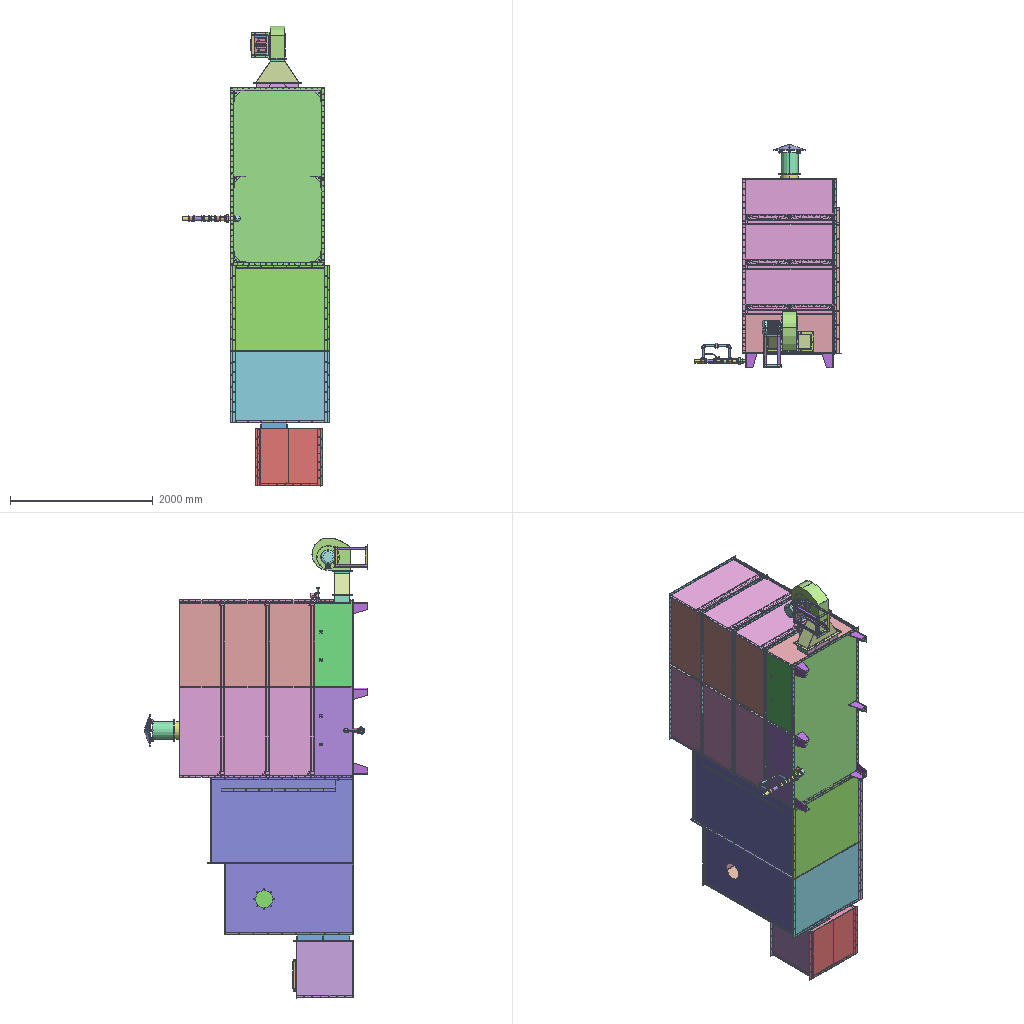Assembly | SolidWorks | 138 different items | 1633 placed | box 2054 x 3134 x 6443 mm
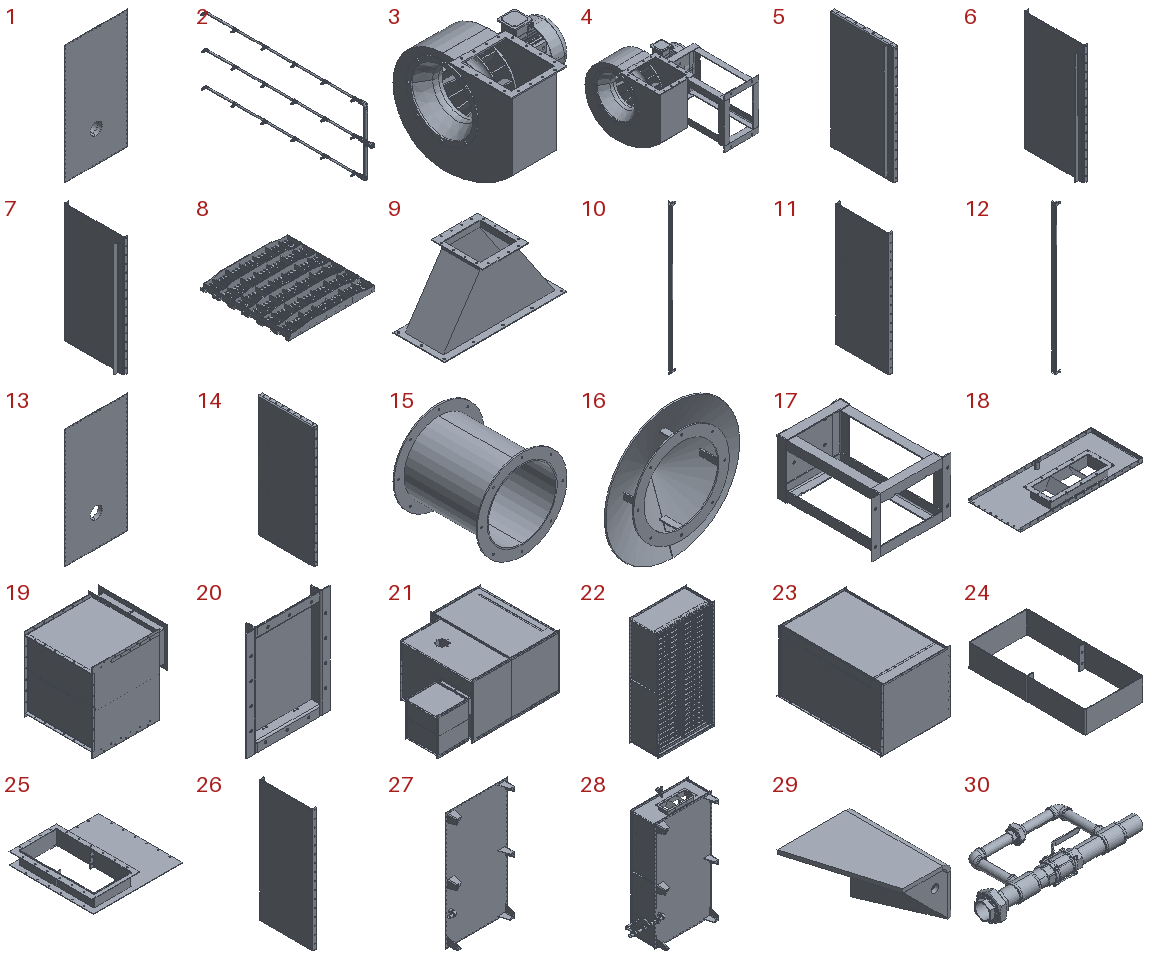Parts list (item | name | quantity | parent item | size | volume | features):
1 | (subassembly) | x1 | - | 1310 x 495.733 x 2490 mm | 15190258 mm3 | features ReferencePattern 45, LocalCirPattern 1, LocalLPattern 1
2 | (subassembly) | x1 | in 28 | 86.11 x 2140 x 858 mm | 1331327 mm3 | features ReferencePattern 36, LocalLPattern 3
3 | (subassembly) | x1 | in 4 | 501 x 560.054 x 460 mm | 9683127 mm3 | -
4 | (subassembly) | x1 | - | 501 x 783.054 x 460 mm | 11094066 mm3 | -
5 | (subassembly) | x6 | in 22 | 80 x 630 x 1180 mm | 3815468 mm3 | -
6 | (subassembly) | x6 | in 22 | 80 x 630 x 1270 mm | 4000203 mm3 | -
7 | (subassembly) | x6 | in 22 | 90 x 630 x 1270 mm | 3990081 mm3 | -
8 | (subassembly) | x24 | in 22 | 610 x 600 x 67 mm | 3647743 mm3 | features ReferencePattern 30, LocalLPattern 2
9 | (subassembly) | x1 | - | 670 x 280 x 338 mm | 2050051 mm3 | -
10 | (subassembly) | x3 | in 22 | 120 x 67 x 2400 mm | 1254438 mm3 | -
11 | (subassembly) | x2 | in 28 | 40 x 540 x 1270 mm | 3162642 mm3 | -
12 | (subassembly) | x6 | in 22 | 77 x 67 x 2400 mm | 1223863 mm3 | -
13 | (subassembly) | x1 | in 1 | 1310 x 80 x 2490 mm | 13192841 mm3 | -
14 | (subassembly) | x2 | in 28 | 40 x 540 x 1180 mm | 3012969 mm3 | -
15 | (subassembly) | x1 | in 1 | 320 x 300 x 320 mm | 1176288 mm3 | -
16 | (subassembly) | x1 | in 1 | 450 x 115.733 x 449.999 mm | 814694 mm3 | -
17 | (subassembly) | x1 | in 4 | 360 x 468 x 250 mm | 1410940 mm3 | -
18 | (subassembly) | x1 | in 28 | 1270 x 540 x 134 mm | 3784835 mm3 | -
19 | (subassembly) | x1 | in 21 | 930 x 849 x 940 mm | 15336660 mm3 | -
20 | (subassembly) | x1 | in 19 | 350 x 43 x 450 mm | 638842 mm3 | -
21 | (subassembly) | x1 | - | 3091 x 2043 x 1380 mm | 102063175 mm3 | features CompositeCurve 1
22 | (subassembly) | x3 | - | - | 57196333 mm3 | features ReferencePattern 7, LocalLPattern 1
23 | (subassembly) | x1 | in 21 | 1380 x 2043 x 1204 mm | 43462479 mm3 | -
24 | (subassembly) | x1 | in 25 | 370 x 740 x 140 mm | 1300830 mm3 | -
25 | (subassembly) | x1 | in 19 | 880 x 840 x 140 mm | 3598044 mm3 | -
26 | (subassembly) | x1 | in 28 | 40 x 540 x 1270 mm | 3163270 mm3 | -
27 | (subassembly) | x1 | in 28 | 1344 x 208 x 2490 mm | 28773491 mm3 | features CompositeCurve 1
28 | (subassembly) | x1 | - | - | 52645263 mm3 | features ReferencePattern 3, LocalLPattern 2
29 | (subassembly) | x6 | in 27 | 160 x 200 x 160 mm | 423977 mm3 | -
30 | (subassembly) | x1 | in 28 | 664 x 302.792 x 119.17 mm | 1293430 mm3 | -
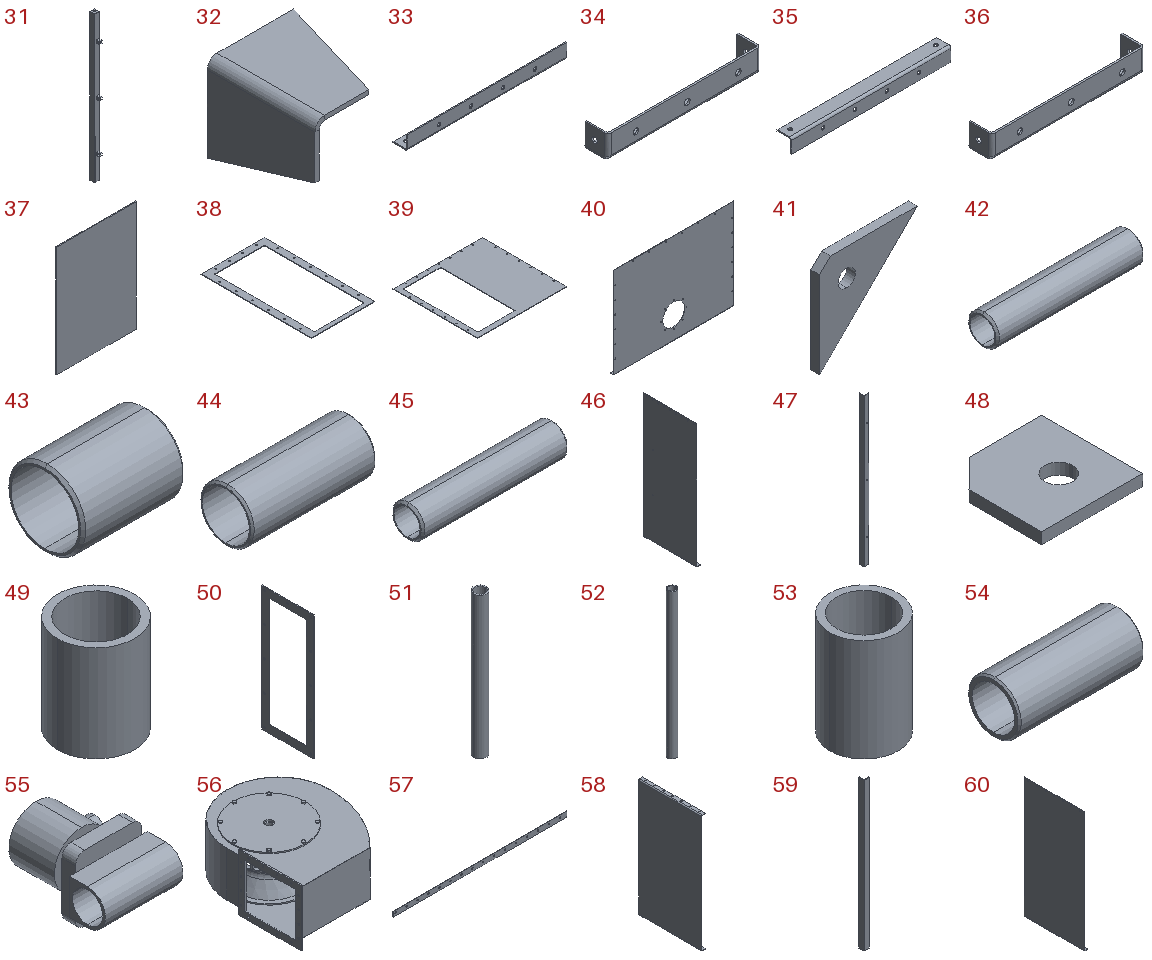31 | (subassembly) | x4 | in 28 | 40 x 68.485 x 1230 mm | 409968 mm3 | -
32 | - | x6 | in 29 | 160 x 200 x 160 mm | 393586 mm3 | features Fillet 2, ICE 2, EdgeFlange 1, FlatPattern 1, SMBaseFlange 1, SheetMetal 1
33 | - | x1 | in 20 | 450 x 40 x 40 mm | 99929 mm3 | features EdgeFlange 1, FlatPattern 1, ICE 1, SMBaseFlange 1, SheetMetal 1
34 | - | x1 | in 20 | 270 x 40 x 40 mm | 67307 mm3 | features CornerFeat 1, EdgeFlange 1, FlatPattern 1, ICE 1, SMBaseFlange 1, SheetMetal 1
35 | - | x1 | in 20 | 450 x 40 x 40 mm | 99929 mm3 | features EdgeFlange 1, FlatPattern 1, ICE 1, SMBaseFlange 1, SheetMetal 1
36 | - | x1 | in 20 | 270 x 40 x 40 mm | 67116 mm3 | features ICE 2, CornerFeat 1, EdgeFlange 1, FlatPattern 1, SMBaseFlange 1, SheetMetal 1
37 | - | x1 | in 20 | 270 x 3 x 376 mm | 304560 mm3 | features FlatPattern 1, SMBaseFlange 1, SheetMetal 1
38 | - | x1 | in 25 | 470 x 820 x 4 mm | 441497 mm3 | features Fillet 1, FlatPattern 1, ICE 1, SMBaseFlange 1, SheetMetal 1
39 | - | x1 | in 25 | 880 x 840 x 4 mm | 1855717 mm3 | features Fillet 1, FlatPattern 1, SMBaseFlange 1, SheetMetal 1
40 | - | x1 | in 21 | 1320 x 40 x 1000 mm | 3955615 mm3 | features ICE 3, CirPattern 1, EdgeFlange 1, FlatPattern 1, RefAxis 1, SMBaseFlange 1, SheetMetal 1
41 | - | x6 | in 29 | 90 x 8 x 90 mm | 30392 mm3 | features Chamfer 1, Extrusion 1, HoleWzd 1
42 | - | x2 | in 30 | 160 x 33.5 x 33.5 mm | 49013 mm3 | features Chamfer 1, ExtruThin 1
43 | - | x1 | in 30 | 80 x 60 x 60 mm | 48963 mm3 | features Chamfer 1, ExtruThin 1
44 | - | x1 | in 30 | 140 x 60 x 60 mm | 86238 mm3 | features Chamfer 1, ExtruThin 1
45 | - | x2 | in 30 | 152 x 33.5 x 33.5 mm | 46542 mm3 | features Chamfer 1, ExtruThin 1
46 | - | x2 | in 11 | 40 x 540 x 1270 mm | 2808187 mm3 | features HoleWzd 3, LPattern 2, EdgeFlange 1, FlatPattern 1, MirrorPattern 1, SMBaseFlange 1, SheetMetal 1, UnFold 1, WeldmentFeature 1
47 | - | x4 | in 31 | 40 x 40 x 1230 mm | 378926 mm3 | features Extrusion 1, HoleWzd 1, LPattern 1
48 | - | x8 | in 31 | 36 x 36 x 4 mm | 4670 mm3 | features Chamfer 1, Extrusion 1, HoleWzd 1
49 | - | x4 | in 2 | 32 x 32 x 40 mm | 10933 mm3 | features ExtruThin 1
50 | - | x2 | in 9, 18 | 4 x 280 x 670 mm | 274630 mm3 | features ExtruThin 1, HoleWzd 1, LPattern 1
51 | - | x2 | in 2 | 32 x 32 x 360 mm | 98395 mm3 | features ExtruThin 1
52 | - | x15 | in 2 | 20 x 20 x 350 mm | 39584 mm3 | features ExtruThin 1
53 | - | x3 | in 2 | 20 x 20 x 30 mm | 3393 mm3 | features ExtruThin 1
54 | - | x1 | in 28 | 80 x 33.5 x 33.5 mm | 24605 mm3 | features Chamfer 1, ExtruThin 1
55 | - | x1 | in 28 | 86 x 120 x 73 mm | 283263 mm3 | features ICE 5, ExtruThin 1
56 | - | x1 | in 3 | 460 x 560.054 x 251 mm | 3395369 mm3 | features Boss 6, Revolution 3, CirPattern 2, Cut 2, Extrusion 1, ICE 1, MirrorPattern 1, RevCut 1, Shell 1
57 | - | x32 | in 6, 7, 11, 18, 26 | 1266 x 4 x 36 mm | 177227 mm3 | features Chamfer 1, Extrusion 1, HoleWzd 1, LPattern 1
58 | - | x6 | in 5 | 40 x 630 x 1180 mm | 3135499 mm3 | features EdgeFlange 1, FlatPattern 1, HoleWzd 1, ICE 1, LPattern 1, SMBaseFlange 1, SheetMetal 1
59 | - | x6 | in 5 | 40 x 40 x 1138 mm | 352057 mm3 | features Extrusion 1
60 | - | x12 | in 6, 7 | 40 x 630 x 1270 mm | 3279151 mm3 | features HoleWzd 2, LPattern 2, EdgeFlange 1, FlatPattern 1, ICE 1, SMBaseFlange 1, SheetMetal 1
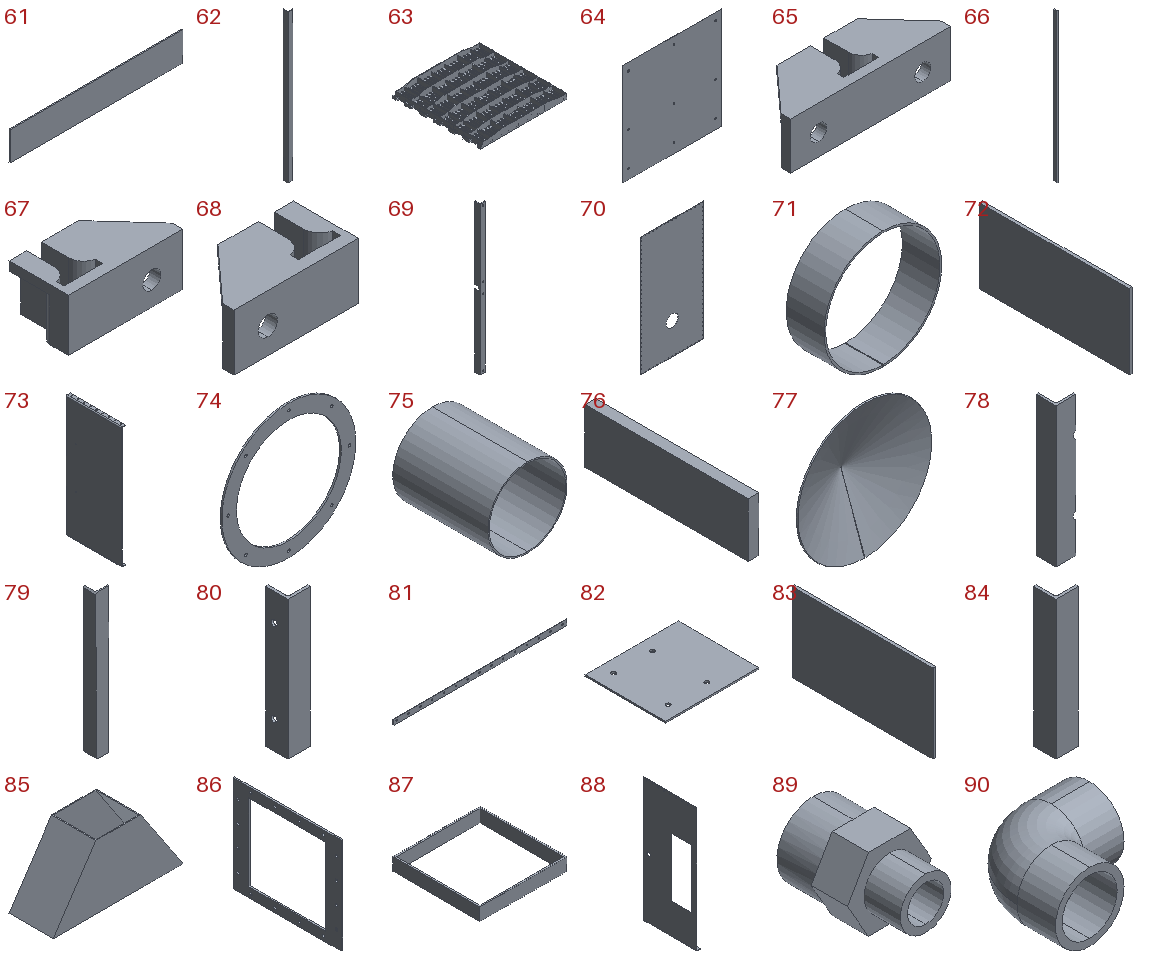61 | - | x2 | in 18 | 600 x 4 x 100 mm | 240000 mm3 | features Extrusion 1
62 | - | x6 | in 6 | 40 x 40 x 1185 mm | 366598 mm3 | features Extrusion 1
63 | - | x24 | in 8 | 610 x 600 x 50 mm | 3519467 mm3 | features ICE 7, LPattern 4, MirrorPattern 4, BossThin 1, Extrusion 1
64 | - | x24 | in 8 | 580 x 0.18 x 600 mm | 62513 mm3 | features LPattern 2, Extrusion 1, FlatPattern 1, HoleWzd 1, SheetMetal 1, SolidToSheetMetal 1
65 | - | x6 | in 10 | 120 x 40 x 35 mm | 52086 mm3 | features ICE 3, Fillet 2, MirrorPattern 2, Extrusion 1
66 | - | x9 | in 10, 12 | 26 x 60 x 2400 mm | 1150265 mm3 | features Fillet 2, Extrusion 1
67 | - | x6 | in 12 | 77 x 40 x 35 mm | 36799 mm3 | features ICE 4, Fillet 2, MirrorPattern 2, Extrusion 1
68 | - | x6 | in 12 | 77 x 40 x 35 mm | 36799 mm3 | features ICE 4, Fillet 2, MirrorPattern 2, Extrusion 1
69 | - | x6 | in 22 | 40 x 40 x 1150 mm | 350360 mm3 | features Extrusion 1, HoleWzd 1, ICE 1
70 | - | x1 | in 13 | 1310 x 4 x 2490 mm | 12821719 mm3 | features CirPattern 2, HoleWzd 2, LPattern 2, Extrusion 1, ICE 1, RefAxis 1
71 | - | x1 | in 13 | 250 x 80 x 249.996 mm | 246676 mm3 | features FlatPattern 1, SheetMetal 1, SweptFlange 1
72 | - | x2 | in 18 | 4 x 200 x 100 mm | 80000 mm3 | features Extrusion 1
73 | - | x2 | in 14 | 40 x 540 x 1180 mm | 2685058 mm3 | features HoleWzd 3, LPattern 2, EdgeFlange 1, FlatPattern 1, MirrorPattern 1, SMBaseFlange 1, SheetMetal 1, UnFold 1, WeldmentFeature 1
74 | - | x4 | in 13, 15, 16 | 320 x 4 x 320 mm | 124445 mm3 | features CirPattern 1, Extrusion 1, ICE 1
75 | - | x1 | in 15 | 250 x 300 x 250 mm | 927398 mm3 | features ExtruThin 1
76 | - | x4 | in 16 | 4 x 60 x 20 mm | 4800 mm3 | features Extrusion 1
77 | - | x1 | in 16 | 450 x 83.765 x 449.999 mm | 671050 mm3 | features FlatPattern 1, LoftedBend 1, SheetMetal 1
78 | - | x4 | in 17 | 40 x 40 x 280 mm | 86131 mm3 | features Cut 1, Extrusion 1
79 | - | x4 | in 17 | 40 x 40 x 456 mm | 140103 mm3 | features Cut 1, Extrusion 1
80 | - | x2 | in 17 | 40 x 40 x 250 mm | 76581 mm3 | features Extrusion 1, HoleWzd 1
81 | - | x16 | in 5, 14 | 1172 x 4 x 36 mm | 163956 mm3 | features Chamfer 1, Extrusion 1, HoleWzd 1, LPattern 1
82 | - | x1 | in 17 | 240 x 208 x 4 mm | 198159 mm3 | features Cut 1, Extrusion 1
83 | - | x2 | in 18 | 4 x 200 x 112 mm | 89600 mm3 | features Extrusion 1
84 | - | x2 | in 17 | 40 x 40 x 250 mm | 77341 mm3 | features Extrusion 1
85 | - | x1 | in 9 | 609.615 x 208 x 300 mm | 1559964 mm3 | features Blend 1
86 | - | x1 | in 9 | 4 x 280 x 250 mm | 117537 mm3 | features Boss 6, ICE 3, Revolution 3, CirPattern 2, Cut 2, Extrusion 1, MirrorPattern 1, RevCut 1, Shell 1
87 | - | x1 | in 9 | 208 x 208 x 30 mm | 97920 mm3 | features ExtruThin 1
88 | - | x1 | in 18 | 40 x 540 x 1270 mm | 2305767 mm3 | features HoleWzd 2, ICE 2, LPattern 2, Cut 1, EdgeFlange 1, FlatPattern 1, SMBaseFlange 1, SheetMetal 1
89 | - | x18 | in 2 | 23.094 x 31 x 20 mm | 4677 mm3 | features BossThin 1, ExtruThin 1, ICE 1
90 | - | x3 | in 2 | 39.5 x 39.5 x 25 mm | 8557 mm3 | features Sweep 1
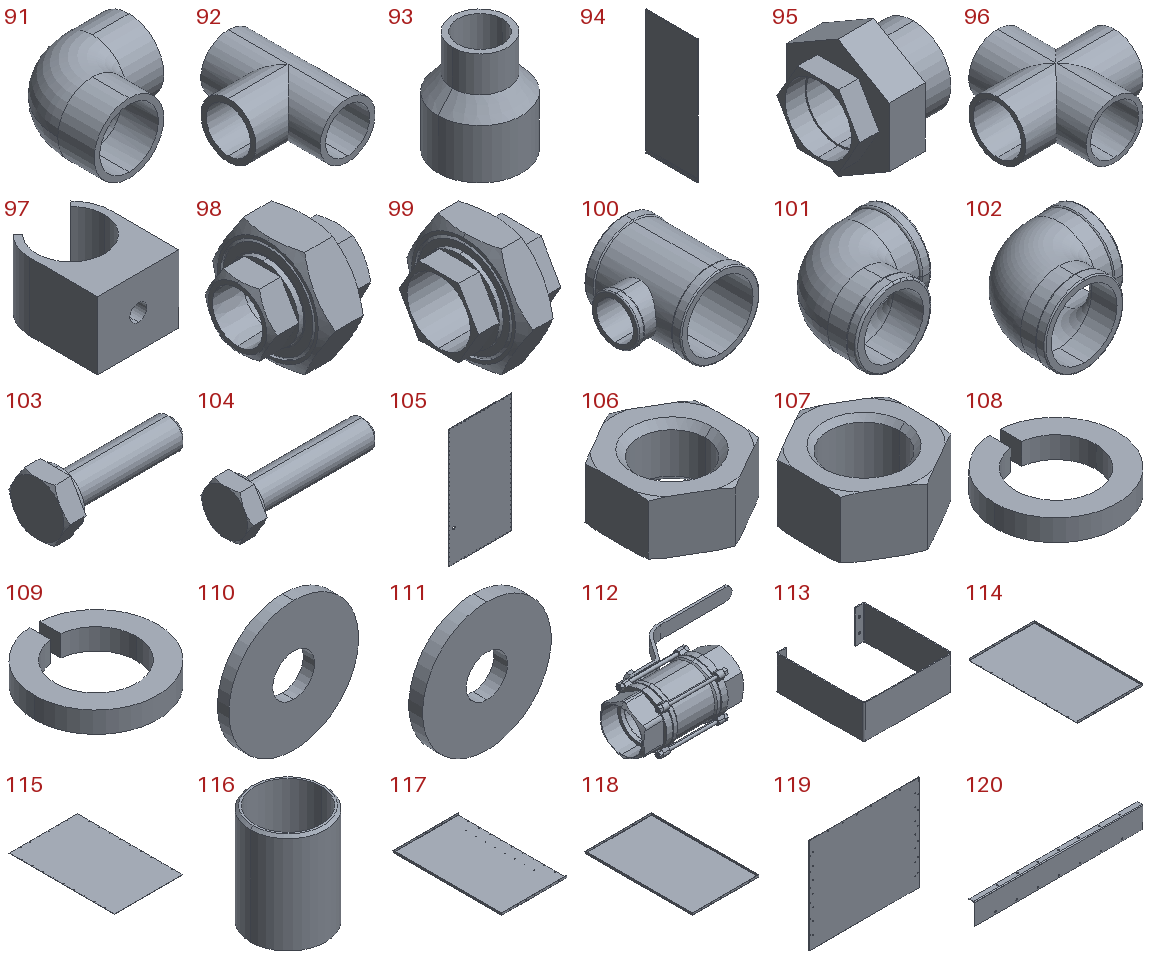91 | - | x2 | in 2 | 59 x 59 x 38 mm | 23558 mm3 | features Sweep 1
92 | - | x15 | in 2 | 39.5 x 54 x 25 mm | 11772 mm3 | features Cut 2, CirPattern 1, RefAxis 1, Revolution 1
93 | - | x3 | in 2 | 38 x 38 x 46 mm | 12125 mm3 | features Revolution 1
94 | - | x1 | in 26 | 4 x 540 x 1303 mm | 2808816 mm3 | features HoleWzd 2, LPattern 2, EdgeFlange 1, FlatPattern 1, SMBaseFlange 1, SheetMetal 1, UnFold 1, WeldmentFeature 1
95 | - | x1 | in 2 | 48 x 51.962 x 60 mm | 36619 mm3 | features ICE 2, ExtruThin 1
96 | - | x1 | in 2 | 78 x 78 x 38 mm | 36723 mm3 | features ICE 2, CirPattern 1, RefAxis 1, Revolution 1
97 | - | x12 | in 31 | 24 x 28.485 x 20 mm | 6832 mm3 | features Extrusion 1, HoleWzd 1, ICE 1
98 | - | x1 | in 30 | 58 x 70.38 x 60.951 mm | 76848 mm3 | features Cut 4, Revolution 3, Chamfer 1, MirrorPattern 1
99 | - | x1 | in 30 | 78 x 119.17 x 103.204 mm | 236540 mm3 | features Cut 3, ICE 3, Revolution 3, MirrorPattern 2, Chamfer 1
100 | - | x2 | in 30 | 88 x 88 x 72 mm | 98463 mm3 | features BossThin 3, Cut 2, Revolution 2, Fillet 1
101 | - | x2 | in 30 | 59.5 x 59.5 x 43 mm | 30865 mm3 | features BossThin 2, Fillet 2, Sweep 1
102 | - | x1 | in 27 | 94 x 94 x 72 mm | 106922 mm3 | features BossThin 2, Fillet 2, Sweep 1
103 | - | x28 | in 1, 31 | 17.8 x 8.083 x 7 mm | 303.684 mm3 | features RevCut 4, Chamfer 1, Extrusion 1, Fillet 1, LPattern 1, Revolution 1
104 | - | x216 | in 8 | 40.3 x 15.011 x 13 mm | 2514 mm3 | features RevCut 4, Chamfer 1, Extrusion 1, Fillet 1, LPattern 1, Revolution 1
105 | - | x1 | in 27 | 1310 x 8 x 2490 mm | 26011985 mm3 | features CirPattern 2, HoleWzd 2, LPattern 2, FlatPattern 1, ICE 1, RefAxis 1, SMBaseFlange 1, SheetMetal 1
106 | - | x28 | in 1, 31 | 6.649 x 7.66 x 3.2 mm | 79.578 mm3 | features Cut 2, Chamfer 1, Extrusion 1
107 | - | x216 | in 8 | 12.482 x 14.38 x 6.8 mm | 562.42 mm3 | features Cut 2, Chamfer 1, Extrusion 1
108 | - | x28 | in 1, 31 | 6.287 x 6.275 x 1.1 mm | 18.963 mm3 | features Extrusion 1
109 | - | x216 | in 8 | 12.277 x 12.254 x 2.1 mm | 135.755 mm3 | features Extrusion 1
110 | - | x216 | in 8 | 34 x 3 x 34 mm | 2439 mm3 | features Revolution 1
111 | - | x216 | in 8 | 28 x 3 x 28 mm | 1656 mm3 | features Revolution 1
112 | - | x1 | in 30 | 259 x 138.2 x 75 mm | 272305 mm3 | features Boss 8, Fillet 5, MirrorPattern 3, RevCut 2, Revolution 2, Chamfer 1, CirPattern 1, Cut 1, ICE 1
113 | - | x2 | in 24 | 370 x 370 x 140 mm | 650415 mm3 | features EdgeFlange 3, FlatPattern 1, ICE 1, SMBaseFlange 1, SheetMetal 1
114 | - | x1 | in 23 | 1200 x 2000 x 40 mm | 7654629 mm3 | features ICE 3, CornerFeat 1, EdgeFlange 1, FlatPattern 1, SMBaseFlange 1, SheetMetal 1
115 | - | x1 | in 23 | 1320 x 2040 x 4 mm | 10763660 mm3 | features FlatPattern 1, SMBaseFlange 1, SheetMetal 1
116 | - | x1 | in 27 | 60 x 60 x 80 mm | 49331 mm3 | features Chamfer 1, Extrusion 1
117 | - | x1 | in 23 | 1200 x 2000 x 40 mm | 7652744 mm3 | features ICE 4, CornerFeat 1, EdgeFlange 1, FlatPattern 1, SMBaseFlange 1, SheetMetal 1
118 | - | x1 | in 23 | 1240 x 2000 x 40 mm | 8113191 mm3 | features ICE 2, CornerFeat 1, EdgeFlange 1, FlatPattern 1, SMBaseFlange 1, SheetMetal 1
119 | - | x1 | in 23 | 1380 x 3 x 1200 mm | 4960460 mm3 | features ICE 2, SMBaseFlange 2, FlatPattern 1, SheetMetal 1
120 | - | x1 | in 23 | 1240 x 40 x 157 mm | 711196 mm3 | features ICE 2, EdgeFlange 1, FlatPattern 1, SMBaseFlange 1, SheetMetal 1
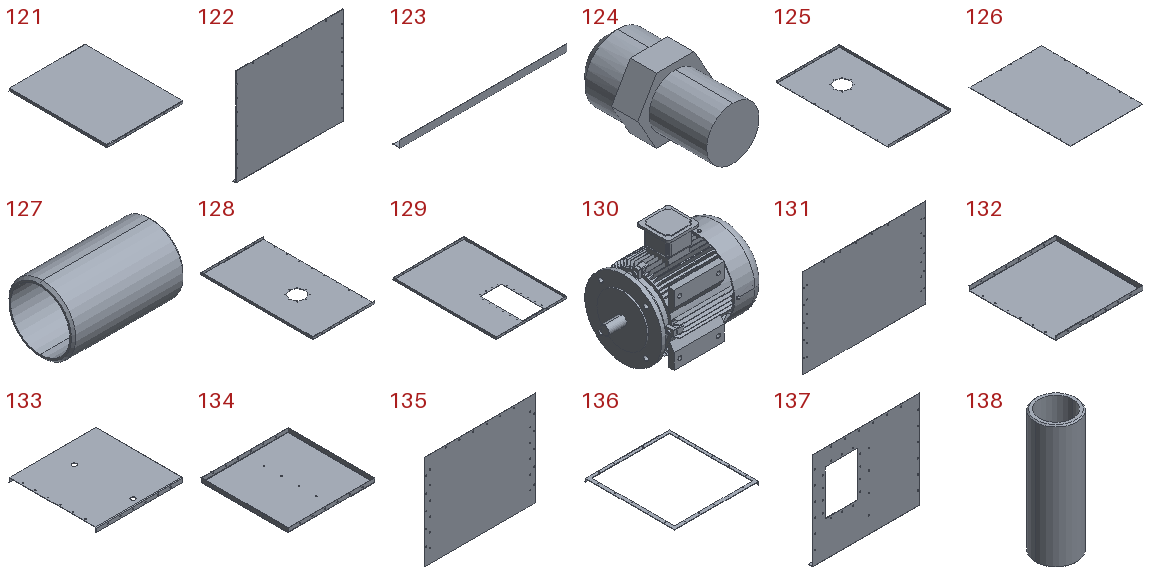121 | - | x1 | in 23 | 1240 x 1600 x 40 mm | 6376482 mm3 | features ICE 2, CornerFeat 1, EdgeFlange 1, FlatPattern 1, SMBaseFlange 1, SheetMetal 1
122 | - | x1 | in 23 | 1320 x 40 x 1200 mm | 4884745 mm3 | features ICE 2, EdgeFlange 1, FlatPattern 1, SMBaseFlange 1, SheetMetal 1
123 | - | x6 | in 7 | 1200 x 50 x 50 mm | 356475 mm3 | features Extrusion 1
124 | - | x18 | in 2 | 14.3 x 24 x 12.384 mm | 2422 mm3 | features ICE 2, Chamfer 1, Extrusion 1
125 | - | x1 | in 21 | 1000 x 1800 x 40 mm | 5654846 mm3 | features ICE 4, CirPattern 1, CornerFeat 1, EdgeFlange 1, FlatPattern 1, RefAxis 1, SMBaseFlange 1, SheetMetal 1
126 | - | x1 | in 21 | 1320 x 1840 x 4 mm | 9708288 mm3 | features FlatPattern 1, SMBaseFlange 1, SheetMetal 1
127 | - | x3 | in 27, 30 | 100 x 60 x 60 mm | 61388 mm3 | features Chamfer 1, ExtruThin 1
128 | - | x1 | in 21 | 1000 x 1800 x 40 mm | 5654846 mm3 | features ICE 4, CirPattern 1, CornerFeat 1, EdgeFlange 1, FlatPattern 1, RefAxis 1, SMBaseFlange 1, SheetMetal 1
129 | - | x1 | in 21 | 1240 x 1800 x 40 mm | 6502410 mm3 | features ICE 3, CornerFeat 1, EdgeFlange 1, FlatPattern 1, RefAxis 1, SMBaseFlange 1, SheetMetal 1
130 | - | x1 | in 3 | 317 x 208.5 x 263.5 mm | 6287758 mm3 | features Boss 18, Cut 6, Revolution 5, CirPattern 4, Fillet 4, Chamfer 3, RevCut 2, 3DProfileFeature 1, LPattern 1, MirrorPattern 1, MoveCopyBody 1
131 | - | x1 | in 21 | 1380 x 3 x 1000 mm | 4133403 mm3 | features ICE 2, SMBaseFlange 2, FlatPattern 1, SheetMetal 1
132 | - | x1 | in 19 | 800 x 800 x 40 mm | 2166122 mm3 | features ICE 3, CornerFeat 2, EdgeFlange 2, FlatPattern 1, SMBaseFlange 1, SheetMetal 1
133 | - | x1 | in 19 | 800 x 800 x 40 mm | 2158563 mm3 | features ICE 4, CornerFeat 1, EdgeFlange 1, FlatPattern 1, SMBaseFlange 1, SheetMetal 1
134 | - | x1 | in 19 | 800 x 800 x 40 mm | 2248588 mm3 | features ICE 3, CornerFeat 1, EdgeFlange 1, FlatPattern 1, SMBaseFlange 1, SheetMetal 1
135 | - | x1 | in 19 | 940 x 3 x 800 mm | 2249403 mm3 | features ICE 3, SMBaseFlange 2, FlatPattern 1, SheetMetal 1
136 | - | x1 | in 19 | 755 x 800 x 30 mm | 382350 mm3 | features ICE 3, EdgeFlange 1, FlatPattern 1, SMBaseFlange 1, SheetMetal 1
137 | - | x1 | in 19 | 880 x 40 x 800 mm | 1894749 mm3 | features ICE 5, EdgeFlange 1, FlatPattern 1, SMBaseFlange 1, SheetMetal 1
138 | - | x1 | in 18 | 33.5 x 33.5 x 100 mm | 30783 mm3 | features Chamfer 2, Extrusion 1
Mates (type | each side: item.copy, entity, surface, feature), first 407 of 559 lines:
In the top assembly
Coincident | 57.1 face plane Boss-Extrude 1 | 57.2 face plane Boss-Extrude 1
Concentric | 57.1 face cylinder Ø10.0 (10) DiameterHole 1 | 57.2 face cylinder Ø10.0 (10) DiameterHole 1
Concentric | 57.1 face cylinder LPattern 1 | 57.2 face cylinder LPattern 1
Coincident | 57.3 face plane Boss-Extrude 1 | 70.1 face plane Boss-Extrude 1
Concentric | 57.4 face cylinder Ø10.0 (10) DiameterHole 1 | 70.1 face cylinder CirPattern 1
Concentric | 57.3 face cylinder LPattern 1 | 70.1 face cylinder CirPattern 1
Concentric | 50.1 face cylinder LPattern 1 | 50.2 face cylinder LPattern 1 | 2 times
Coincident | 50.1 face plane Extrude-Thin-Wall 1 | 50.2 face plane Extrude-Thin-Wall 1
Coincident | 56.1 face plane Extrude 2 | 86.1 face plane Extrude 2
Concentric | 56.1 face cylinder Cut-Extrude 5 | 86.1 face cylinder Cut-Extrude 5 | 2 times
Coincident | 105.1 face plane Base-Flange 1 | 119.1 face plane Base-Flange 1 | 2 times
Coincident | 105.1 face plane Base-Flange 1 | 119.1 face plane Sheet 1
In subassembly 22
Coincident | 58.1 face plane Edge-Flange 2 | 60.1 face plane Edge-Flange 2
Concentric | 58.1 face cylinder Ø10.0 (10) DiameterHole 3 | 60.1 face cylinder Ø10.0 (10) DiameterHole 3
Concentric | 58.1 face cylinder LPattern 5 | 60.1 face cylinder LPattern 5
Coincident | 60.1 face plane Base-Flange 1 | 60.2 face plane Edge-Flange 2
Concentric | 60.1 face cylinder Ø10.0 (10) DiameterHole 2 | 60.2 face cylinder Ø10.0 (10) DiameterHole 3
Concentric | 60.1 face cylinder LPattern 3 | 60.2 face cylinder LPattern 5
Coincident | 60.2 face plane Base-Flange 1 | 58.2 face plane Edge-Flange 2
Concentric | 60.2 face cylinder Ø10.0 (10) DiameterHole 2 | 58.2 face cylinder Ø10.0 (10) DiameterHole 3
Concentric | 60.2 face cylinder LPattern 3 | 58.2 face cylinder LPattern 5
Coincident | 58.2 face plane Edge-Flange 2 | 60.3 face plane Edge-Flange 2
Concentric | 58.2 face cylinder Ø10.0 (10) DiameterHole 3 | 60.3 face cylinder Ø10.0 (10) DiameterHole 3
Concentric | 58.2 face cylinder LPattern 5 | 60.3 face cylinder LPattern 5
Coincident | 60.3 face plane Base-Flange 1 | 60.4 face plane Edge-Flange 2
Concentric | 60.3 face cylinder Ø10.0 (10) DiameterHole 2 | 60.4 face cylinder Ø10.0 (10) DiameterHole 3
Concentric | 60.3 face cylinder LPattern 3 | 60.4 face cylinder LPattern 5
Coincident | 123.1 face plane Base | 65.1 face plane Boss-Extrude 1
Coincident | 63.1 face plane Boss-Extrude 1 | 66.1 face plane Boss-Extrude 1
Coincident | 63.2 face plane Boss-Extrude 1 | 66.1 face plane Boss-Extrude 1
Width | 66.1 face plane Boss-Extrude 1 | 66.1 face plane Boss-Extrude 1 | 63.3 face plane Boss-Extrude 1 | 63.4 face plane Boss-Extrude 1
Coincident | 123.1 face plane Base | 68.1 face plane Boss-Extrude 1
Coincident | 123.1 face plane Base | 67.1 face plane Boss-Extrude 1
Coincident | 123.2 face plane Base | 69.1 face plane Extrude 1
Coincident | 123.1 face plane Base | 69.2 face plane Extrude 1
In subassembly 8
Coincident | 63.5 face plane Boss-Extrude 1 | 64.1 face plane Convert Body 1 | 3 times
Coincident | 63.5 face plane Boss-Extrude 1 | 111.1 face plane Base-Revolve | 2 times
Coincident | 109.1 face plane Extrude 1 | 111.1 face plane Base-Revolve | 2 times
Coincident | 109.1 face plane Extrude 1 | 107.1 face plane Base-Extrude | 2 times
Coincident | 63.5 axis | 104.1 axis
Coincident | 63.5 axis | 111.1 axis
Coincident | 109.2 face plane Extrude 1 | 111.2 face plane Base-Revolve | 2 times
Coincident | 109.2 face plane Extrude 1 | 107.2 face plane Base-Extrude | 2 times
Coincident | 63.5 face plane Boss-Extrude 1 | 111.2 face plane Base-Revolve | 2 times
Coincident | 63.5 axis | 111.2 axis
Coincident | 109.3 face plane Extrude 1 | 111.3 face plane Base-Revolve | 2 times
Coincident | 109.3 face plane Extrude 1 | 107.3 face plane Base-Extrude | 2 times
Coincident | 63.5 face plane Boss-Extrude 1 | 111.3 face plane Base-Revolve | 2 times
Coincident | 63.5 axis | 111.3 axis
Coincident | 104.1 axis | 110.1 axis
Coincident | 104.1 face plane Base-Extrude | 110.1 face plane Base-Revolve
Coincident | 63.5 face plane Boss-Extrude 6 | 110.1 face plane Base-Revolve
Coincident | 104.1 axis | 109.1 axis
Coincident | 104.1 axis | 107.1 axis
Coincident | 104.2 axis | 110.2 axis
Coincident | 104.2 face plane Base-Extrude | 110.2 face plane Base-Revolve
Coincident | 63.5 axis | 104.2 axis
Coincident | 63.5 face plane LPattern 4 | 110.2 face plane Base-Revolve
Coincident | 104.2 axis | 109.2 axis
Coincident | 104.2 axis | 107.2 axis
Coincident | 104.3 axis | 110.3 axis
Coincident | 104.3 face plane Base-Extrude | 110.3 face plane Base-Revolve
Coincident | 63.5 axis | 104.3 axis
Coincident | 63.5 face plane LPattern 4 | 110.3 face plane Base-Revolve
Coincident | 104.3 axis | 109.3 axis
Coincident | 104.3 axis | 107.3 axis
Parallel | 104.1 face plane Base-Extrude | 8.1 plane
Parallel | 104.2 face plane Base-Extrude | 8.1 plane
Parallel | 104.3 face plane Base-Extrude | 8.1 plane
Parallel | 107.3 face plane Base-Extrude | 8.1 plane
Parallel | 107.2 face plane Base-Extrude | 8.1 plane
Parallel | 107.1 face plane Base-Extrude | 8.1 plane
In subassembly 5
Coincident | 58.3 face plane Base-Flange 1 | 81.1 face plane Boss-Extrude 1 | 2 times
Coincident | 58.3 face plane Edge-Flange 2 | 81.1 face plane Boss-Extrude 1
Coincident | 58.3 face plane Base-Flange 1 | 81.2 face plane Boss-Extrude 1 | 2 times
Coincident | 58.3 face plane Edge-Flange 2 | 81.2 face plane Boss-Extrude 1
Coincident | 58.3 face plane Base-Flange 1 | 59.1 face plane Extrude 1
Coincident | 58.3 face plane Edge-Flange 2 | 59.1 face plane Extrude 1
DistanceDim | 59.1 face plane Extrude 1 | 58.3 face plane Base-Flange 1
In subassembly 6
Coincident | 60.5 face plane Edge-Flange 2 | 57.5 face plane Boss-Extrude 1
Coincident | 60.5 face plane Base-Flange 1 | 57.5 face plane Boss-Extrude 1 | 2 times
Coincident | 60.5 face plane Edge-Flange 2 | 57.6 face plane Boss-Extrude 1
Coincident | 60.5 face plane Base-Flange 1 | 57.6 face plane Boss-Extrude 1 | 2 times
Coincident | 60.5 face plane Base-Flange 1 | 62.1 face plane Extrude 1
Coincident | 60.5 face plane Edge-Flange 2 | 62.1 face plane Extrude 1
DistanceDim | 62.1 face plane Extrude 1 | 60.5 face plane Base-Flange 1
In subassembly 7
Coincident | 60.5 face plane Edge-Flange 2 | 57.5 face plane Boss-Extrude 1
Coincident | 60.5 face plane Base-Flange 1 | 57.5 face plane Boss-Extrude 1 | 2 times
Coincident | 60.5 face plane Edge-Flange 2 | 57.6 face plane Boss-Extrude 1
Coincident | 60.5 face plane Base-Flange 1 | 57.6 face plane Boss-Extrude 1 | 2 times
Coincident | 60.5 face plane Base-Flange 1 | 123.3 face plane Base
Coincident | 123.3 face plane Base | 60.5 face plane Edge-Flange 2
DistanceDim | 123.3 face plane Base | 60.5 face plane Base-Flange 1
In subassembly 10
Coincident | 65.2 plane | 66.2 plane
Coincident | 65.2 face plane Boss-Extrude 1 | 66.2 face plane Boss-Extrude 1
Coincident | 66.2 face plane Boss-Extrude 1 | 65.3 face plane Boss-Extrude 1 | 2 times
Coincident | 66.2 plane | 65.3 plane
DistanceDim | 65.2 face cylinder Cut-Extrude 1 | 65.3 face cylinder Mirror 2
In subassembly 12
DistanceDim | 67.2 axis | 68.2 axis
Coincident | 66.2 face plane Boss-Extrude 1 | 67.2 face plane Boss-Extrude 1
Coincident | 66.2 face plane Boss-Extrude 1 | 68.2 face plane Boss-Extrude 1 | 2 times
Coincident | 66.2 plane | 67.2 plane
Coincident | 66.2 plane | 68.2 plane
In subassembly 1
Coincident | 74.1 face plane Boss-Extrude 1 | 74.2 face plane Boss-Extrude 1
Coincident | 74.1 axis | 74.2 axis | 2 times
Coincident | 74.1 axis | 103.1 axis
Coincident | 74.2 face plane Boss-Extrude 1 | 103.1 face plane Base-Extrude
Coincident | 103.1 axis | 108.1 axis
Coincident | 74.1 face plane Boss-Extrude 1 | 108.1 face plane Extrude 1
Coincident | 103.1 axis | 106.1 axis
Coincident | 108.1 face plane Extrude 1 | 106.1 face plane Base-Extrude
Coincident | 75.1 axis | 74.3 axis
Coincident | 74.4 axis | 74.3 axis
Coincident | 74.4 face plane Boss-Extrude 1 | 74.3 face plane Boss-Extrude 1
In subassembly 15
Coincident | 75.2 axis | 74.5 axis
Coincident | 75.2 face plane Extrude-Thin-Wall 1 | 74.5 face plane Boss-Extrude 1
Coincident | 75.2 axis | 74.6 axis
Coincident | 75.2 face plane Extrude-Thin-Wall 1 | 74.6 face plane Boss-Extrude 1
In subassembly 13
Concentric | 70.2 face cylinder Cut-Extrude 1 | 71.1 face cylinder SweepFlange 1
Coincident | 70.2 face plane Boss-Extrude 1 | 71.1 face plane Sweep Bend 1_1
Concentric | 71.1 face cylinder SweepFlange 1 | 74.5 face cylinder Boss-Extrude 1
Coincident | 71.1 face plane Sweep Bend 1_1 | 74.5 face plane Boss-Extrude 1
In subassembly 16
Coincident | 74.5 plane | 76.1 face plane Boss-Extrude 1
Coincident | 74.5 face plane Boss-Extrude 1 | 76.1 face plane Boss-Extrude 1
DistanceDim | 76.1 face plane Boss-Extrude 1 | 74.5 plane
Coincident | 74.5 plane | 76.2 face plane Boss-Extrude 1
Coincident | 74.5 face plane Boss-Extrude 1 | 76.2 face plane Boss-Extrude 1
DistanceDim | 76.2 face plane Boss-Extrude 1 | 74.5 plane
Coincident | 74.5 plane | 76.3 face plane Boss-Extrude 1
Coincident | 74.5 face plane Boss-Extrude 1 | 76.3 face plane Boss-Extrude 1
DistanceDim | 76.3 face plane Boss-Extrude 1 | 74.5 plane
Coincident | 74.5 plane | 76.4 face plane Boss-Extrude 1
Coincident | 74.5 face plane Boss-Extrude 1 | 76.4 face plane Boss-Extrude 1
DistanceDim | 76.4 face plane Boss-Extrude 1 | 74.5 plane
Coincident | 77.1 plane | 16.1 plane | 2 times
Coincident | 76.4 vertex | 77.1 face cone Freeform Bend 1
In subassembly 9
Coincident | 85.1 face plane Loft-Thin Feature 1 | 50.3 face plane Extrude-Thin-Wall 1
Coincident | 85.1 plane | 50.3 plane | 2 times
Coincident | 85.1 plane | 86.2 plane | 2 times
Coincident | 85.1 plane | 87.1 plane | 2 times
Coincident | 85.1 face plane Loft-Thin Feature 1 | 87.1 face plane Extrude-Thin-Wall 1
Coincident | 86.2 face plane Extrude 2 | 87.1 face plane Extrude-Thin-Wall 1
In subassembly 28
Coincident | 46.1 face plane Edge-Flange 2 | 73.1 face plane Edge-Flange 2
Concentric | 46.1 face cylinder Ø10.0 (10) DiameterHole 2 | 73.1 face cylinder Ø10.0 (10) DiameterHole 4
Concentric | 46.1 face cylinder LPattern 2 | 73.1 face cylinder LPattern 3
Coincident | 46.1 face plane Base-Flange 1 | 88.1 face plane Edge-Flange 2
Concentric | 46.1 face cylinder Ø10.0 (10) DiameterHole 1 | 88.1 face cylinder Ø10.0 (10) DiameterHole 2
Concentric | 46.1 face cylinder LPattern 1 | 88.1 face cylinder LPattern 2
Coincident | 88.1 face plane Base-Flange 1 | 73.2 face plane Edge-Flange 2
Concentric | 88.1 face cylinder Ø10.0 (10) DiameterHole 1 | 73.2 face cylinder Ø10.0 (10) DiameterHole 2
Concentric | 88.1 face cylinder LPattern 1 | 73.2 face cylinder LPattern 2
Coincident | 73.2 face plane Edge-Flange 2 | 46.2 face plane Edge-Flange 2
Concentric | 73.2 face cylinder Ø10.0 (10) DiameterHole 4 | 46.2 face cylinder Ø10.0 (10) DiameterHole 2
Concentric | 73.2 face cylinder LPattern 3 | 46.2 face cylinder LPattern 2
Coincident | 94.1 face plane Edge-Flange 2 | 46.2 face plane Base-Flange 1
Concentric | 94.1 face cylinder Ø10.0 (10) DiameterHole 2 | 46.2 face cylinder Ø10.0 (10) DiameterHole 1
Concentric | 94.1 face cylinder LPattern 2 | 46.2 face cylinder LPattern 1
Concentric | 127.1 face cylinder Extrude-Thin-Wall 1 | 99.1 face cylinder Cut-Extrude 5
DistanceDim | 127.1 face plane Extrude-Thin-Wall 1 | 99.1 face plane Revolve 1
Parallel | 105.2 face plane Base-Flange 1 | 30.1 plane
Coincident | 57.7 face plane Boss-Extrude 1 | 105.2 face plane Base-Flange 1
Concentric | 57.7 face cylinder Ø10.0 (10) DiameterHole 1 | 105.2 face cylinder CirPattern 2
Concentric | 57.7 face cylinder LPattern 1 | 105.2 face cylinder CirPattern 2
Coincident | 46.1 face plane Base-Flange 1 | 48.1 face plane Boss-Extrude 1
Concentric | 46.1 face cylinder Mirror 1 | 48.1 face cylinder Ø10.0 (10) DiameterHole 1
Parallel | 46.1 face plane Base-Flange 1 | 47.1 face plane Extrude 1
Concentric | 138.1 face cylinder Boss-Extrude 1 | 95.1 face cylinder Boss-Extrude 2
DistanceDim | 95.1 face plane Boss-Extrude 2 | 138.1 face plane Boss-Extrude 1
Concentric | 97.1 face cylinder Boss-Extrude 1 | 52.1 face cylinder Extrude-Thin-Wall 1
Concentric | 138.1 face cylinder Boss-Extrude 1 | 55.1 face cylinder Extrude-Thin-Wall 1
DistanceDim | 138.1 face plane Boss-Extrude 1 | 55.1 face plane Extrude-Thin-Wall 1
Concentric | 54.1 face cylinder Extrude-Thin-Wall 1 | 55.1 face cylinder Extrude-Thin-Wall 1
DistanceDim | 55.1 face plane Extrude-Thin-Wall 1 | 54.1 face plane Extrude-Thin-Wall 1
Parallel | 46.1 face plane Base-Flange 1 | 55.1 face plane Boss-Extrude 1
In subassembly 31
Coincident | 47.2 face plane Extrude 1 | 48.2 face plane Boss-Extrude 1 | 3 times
Coincident | 47.2 face plane Extrude 1 | 48.3 face plane Boss-Extrude 1 | 3 times
Coincident | 47.2 axis | 97.2 axis
Coincident | 47.2 face plane Extrude 1 | 97.2 face plane Boss-Extrude 1
Parallel | 47.2 face plane Extrude 1 | 97.2 face plane Boss-Extrude 1
Coincident | 47.2 axis | 103.1 axis
Coincident | 97.2 face plane Cut-Extrude 3 | 103.1 face plane Base-Extrude
Coincident | 103.1 axis | 108.1 axis
Coincident | 47.2 face plane Extrude 1 | 108.1 face plane Extrude 1
Coincident | 103.1 axis | 106.1 axis
Coincident | 108.1 face plane Extrude 1 | 106.1 face plane Base-Extrude
Coincident | 97.3 face plane Cut-Extrude 3 | 103.2 face plane Base-Extrude
Coincident | 103.2 axis | 108.2 axis
Coincident | 103.2 axis | 106.2 axis
Coincident | 108.2 face plane Extrude 1 | 106.2 face plane Base-Extrude
Coincident | 47.2 axis | 97.3 axis
Coincident | 47.2 face plane Extrude 1 | 97.3 face plane Boss-Extrude 1
Parallel | 47.2 face plane Extrude 1 | 97.3 face plane Boss-Extrude 1
Coincident | 47.2 axis | 103.2 axis
Coincident | 47.2 face plane Extrude 1 | 108.2 face plane Extrude 1
Coincident | 97.4 face plane Cut-Extrude 3 | 103.3 face plane Base-Extrude
Coincident | 103.3 axis | 108.3 axis
Coincident | 103.3 axis | 106.3 axis
Coincident | 108.3 face plane Extrude 1 | 106.3 face plane Base-Extrude
Coincident | 47.2 axis | 97.4 axis
Coincident | 47.2 face plane Extrude 1 | 97.4 face plane Boss-Extrude 1
Parallel | 47.2 face plane Extrude 1 | 97.4 face plane Boss-Extrude 1
Coincident | 47.2 face plane Extrude 1 | 108.3 face plane Extrude 1
Coincident | 47.2 axis | 103.3 axis
Parallel | 97.4 face plane Cut-Extrude 3 | 103.3 face plane Base-Extrude
Parallel | 97.3 face plane Cut-Extrude 3 | 103.2 face plane Base-Extrude
Parallel | 97.2 face plane Cut-Extrude 3 | 103.1 face plane Base-Extrude
In subassembly 11
Coincident | 46.3 face plane Edge-Flange 2 | 57.5 face plane Boss-Extrude 1
Coincident | 46.3 face plane Base-Flange 1 | 57.5 face plane Boss-Extrude 1 | 2 times
Coincident | 46.3 face plane Base-Flange 1 | 57.6 face plane Boss-Extrude 1 | 2 times
Coincident | 46.3 face plane Edge-Flange 2 | 57.6 face plane Boss-Extrude 1
In subassembly 14
Coincident | 73.3 face plane Base-Flange 1 | 81.1 face plane Boss-Extrude 1 | 2 times
Coincident | 73.3 face plane Edge-Flange 2 | 81.1 face plane Boss-Extrude 1
Coincident | 73.3 face plane Base-Flange 1 | 81.2 face plane Boss-Extrude 1 | 2 times
Coincident | 73.3 face plane Edge-Flange 2 | 81.2 face plane Boss-Extrude 1
In subassembly 27
Coincident | 105.3 face plane Base-Flange 1 | 116.1 edge
Coincident | 116.1 axis | 102.1 axis
DistanceDim | 102.1 face plane Sweep 1 | 116.1 face plane Extrude 1
Coincident | 105.3 axis | 116.1 axis
Coincident | 105.3 face plane Base-Flange 1 | 116.1 face plane Extrude 1
Parallel | 105.3 face plane Base-Flange 1 | 102.1 axis
Coincident | 102.1 axis | 127.2 axis
DistanceDim | 127.2 face plane Extrude-Thin-Wall 1 | 102.1 face plane Sweep 1
Coincident | 105.3 face plane Base-Flange 1 | 32.1 face plane Base-Flange 1
DistanceDim | 32.1 face plane Edge-Flange 1 | 105.3 face plane Base-Flange 1
DistanceDim | 32.1 face plane Base-Flange 1 | 105.3 face plane Base-Flange 1
Coincident | 105.3 face plane Base-Flange 1 | 32.2 face plane Base-Flange 1
DistanceDim | 32.2 face plane Edge-Flange 1 | 105.3 face plane Base-Flange 1
DistanceDim | 32.2 face plane Base-Flange 1 | 105.3 face plane Base-Flange 1
Coincident | 105.3 face plane Base-Flange 1 | 32.3 face plane Base-Flange 1
DistanceDim | 32.3 face plane Edge-Flange 1 | 105.3 face plane Base-Flange 1
DistanceDim | 32.3 face plane Base-Flange 1 | 105.3 face plane Base-Flange 1
Coincident | 105.3 face plane Base-Flange 1 | 32.4 face plane Base-Flange 1
DistanceDim | 32.4 face plane Edge-Flange 1 | 105.3 face plane Base-Flange 1
DistanceDim | 32.4 face plane Base-Flange 1 | 105.3 face plane Base-Flange 1
Coincident | 105.3 face plane Base-Flange 1 | 32.5 face plane Base-Flange 1
DistanceDim | 32.5 face plane Edge-Flange 1 | 105.3 face plane Base-Flange 1
DistanceDim | 32.1 face plane Base-Flange 1 | 32.5 face plane Base-Flange 1
Coincident | 105.3 face plane Base-Flange 1 | 32.6 face plane Base-Flange 1
DistanceDim | 32.6 face plane Base-Flange 1 | 105.3 face plane Base-Flange 1
DistanceDim | 32.6 face plane Edge-Flange 1 | 32.2 face plane Edge-Flange 1
In subassembly 29
Coincident | 32.7 face plane Edge-Flange 1 | 41.1 face plane Boss-Extrude 1
Coincident | 32.7 face plane Base-Flange 1 | 41.1 face plane Boss-Extrude 1 | 2 times
In subassembly 30
Coincident | 43.1 axis | 112.1 axis
Coincident | 42.1 axis | 101.1 axis | 2 times
DistanceDim | 43.1 face plane Extrude-Thin-Wall 1 | 112.1 face plane Revolve 1
Coincident | 112.1 axis | 44.1 axis
DistanceDim | 112.1 face plane Revolve 1 | 44.1 face plane Extrude-Thin-Wall 1
Coincident | 44.1 axis | 100.1 axis
DistanceDim | 100.1 face plane Revolve 1 | 44.1 face plane Extrude-Thin-Wall 1
Parallel | 42.1 axis | 101.2 face cylinder Sweep 1
Coincident | 101.2 axis | 42.2 axis
DistanceDim | 101.2 face plane Sweep 1 | 42.2 face plane Extrude-Thin-Wall 1
Coincident | 100.1 axis | 127.3 axis
DistanceDim | 100.1 face plane Revolve 1 | 127.3 face plane Extrude-Thin-Wall 1
Coincident | 100.1 axis | 42.2 axis
DistanceDim | 42.2 face plane Extrude-Thin-Wall 1 | 100.1 face plane Revolve 2
Coincident | 100.2 plane | 30.2 plane | 3 times
Parallel | 100.1 plane | 30.2 plane
Coincident | 101.2 plane | 30.2 plane
Coincident | 100.2 axis | 43.1 axis
DistanceDim | 100.2 face plane Revolve 1 | 43.1 face plane Extrude-Thin-Wall 1
Coincident | 127.4 axis | 99.2 axis
DistanceDim | 127.4 face plane Extrude-Thin-Wall 1 | 99.2 face plane Revolve 1
Coincident | 127.4 axis | 100.2 axis
DistanceDim | 100.2 face plane Revolve 1 | 127.4 face plane Extrude-Thin-Wall 1
Coincident | 98.1 axis | 45.1 axis
Coincident | 98.1 axis | 45.2 axis
DistanceDim | 98.1 face plane Revolve 1 | 45.1 face plane Extrude-Thin-Wall 1
DistanceDim | 98.1 face plane Revolve 1 | 45.2 face plane Extrude-Thin-Wall 1
Coincident | 101.1 axis | 45.2 axis
DistanceDim | 101.1 face plane Sweep 1 | 45.2 face plane Extrude-Thin-Wall 1
Parallel | 99.2 face plane Cut-Extrude 3 | 30.2 plane
Parallel | 98.1 face plane Cut-Extrude 3 | 30.2 plane
DistanceDim | 42.1 face plane Extrude-Thin-Wall 1 | 100.2 face plane Revolve 2
Coincident | 100.2 axis | 42.1 axis
DistanceDim | 42.1 face plane Extrude-Thin-Wall 1 | 101.1 face plane Sweep 1
In subassembly 18
Coincident | 88.2 face plane Edge-Flange 2 | 57.8 face plane Boss-Extrude 1
Coincident | 88.2 face plane Base-Flange 1 | 57.8 face plane Boss-Extrude 1 | 2 times
DistanceDim | 138.2 face plane Boss-Extrude 1 | 88.2 face plane Base-Flange 1
Coincident | 88.2 face plane Base-Flange 1 | 57.9 face plane Boss-Extrude 1 | 2 times
Coincident | 88.2 face plane Edge-Flange 2 | 57.9 face plane Boss-Extrude 1
Coincident | 88.2 plane | 18.1 plane | 3 times
Coincident | 88.2 axis | 138.2 axis
Coincident | 61.1 face plane Boss-Extrude 1 | 72.1 face plane Boss-Extrude 1 | 3 times
Coincident | 61.1 face plane Boss-Extrude 1 | 72.2 face plane Boss-Extrude 1 | 3 times
Coincident | 61.1 face plane Boss-Extrude 1 | 83.1 face plane Boss-Extrude 1
Coincident | 61.1 face plane Boss-Extrude 1 | 83.2 face plane Boss-Extrude 1
Coincident | 72.1 face plane Boss-Extrude 1 | 61.2 face plane Boss-Extrude 1 | 3 times
DistanceDim | 83.1 edge | 72.1 face plane Boss-Extrude 1 | 2 times
DistanceDim | 83.2 edge | 72.2 face plane Boss-Extrude 1 | 2 times
Coincident | 61.2 face plane Boss-Extrude 1 | 83.1 edge
Coincident | 61.2 face plane Boss-Extrude 1 | 83.2 edge
Coincident | 88.2 face plane Base-Flange 1 | 61.1 face plane Boss-Extrude 1
Coincident | 88.2 face plane Cut-Extrude 2 | 61.1 face plane Boss-Extrude 1 | 2 times
Coincident | 50.4 face plane Extrude-Thin-Wall 1 | 61.1 face plane Boss-Extrude 1 | 2 times
DistanceDim | 50.4 face plane Extrude-Thin-Wall 1 | 72.2 face plane Boss-Extrude 1
In subassembly 26
Coincident | 94.2 face plane Edge-Flange 2 | 57.8 face plane Boss-Extrude 1
Coincident | 94.2 face plane Base-Flange 1 | 57.8 face plane Boss-Extrude 1 | 2 times
Coincident | 94.2 face plane Base-Flange 1 | 57.9 face plane Boss-Extrude 1 | 2 times
Coincident | 94.2 face plane Edge-Flange 2 | 57.9 face plane Boss-Extrude 1
In subassembly 2
Coincident | 49.1 axis | 96.1 axis
DistanceDim | 96.1 face plane CirPattern 1 | 49.1 face plane Extrude-Thin-Wall 1
Coincident | 96.1 axis | 51.1 axis
DistanceDim | 96.1 face plane Revolve 1 | 51.1 face plane Extrude-Thin-Wall 1
Coincident | 96.1 axis | 51.2 axis
DistanceDim | 96.1 face plane CirPattern 1 | 51.2 face plane Extrude-Thin-Wall 1
Coincident | 51.2 axis | 91.1 axis
DistanceDim | 51.2 face plane Extrude-Thin-Wall 1 | 91.1 face plane Sweep 1
Coincident | 51.1 axis | 91.2 axis
DistanceDim | 51.1 face plane Extrude-Thin-Wall 1 | 91.2 face plane Sweep 1
Parallel | 91.1 axis | 2.1 plane
Parallel | 91.2 axis | 2.1 plane
Coincident | 49.1 axis | 95.2 axis
DistanceDim | 49.1 face plane Extrude-Thin-Wall 1 | 95.2 face plane Extrude-Thin-Wall 1
Parallel | 51.2 axis | 2.1 plane | 2 times
Parallel | 96.1 plane | 2.1 plane
Coincident | 92.1 axis | 89.1 axis
DistanceDim | 89.1 face plane Extrude-Thin-Wall 1 | 92.1 face plane CirPattern 1
Coincident | 92.1 axis | 52.2 axis
DistanceDim | 52.2 face plane Extrude-Thin-Wall 1 | 92.1 face plane Revolve 1
Coincident | 92.1 axis | 53.1 axis
DistanceDim | 92.1 face plane CirPattern 1 | 53.1 face plane Extrude-Thin-Wall 1
Coincident | 52.3 axis | 90.1 axis
DistanceDim | 52.3 face plane Extrude-Thin-Wall 1 | 90.1 face plane Sweep 1
DistanceDim | 52.3 face plane Extrude-Thin-Wall 1 | 92.2 face plane Revolve 1
Coincident | 52.3 axis | 92.2 axis
Coincident | 90.1 axis | 89.2 axis
DistanceDim | 89.2 face plane Extrude-Thin-Wall 1 | 90.1 face plane Sweep 1
Coincident | 89.2 axis | 124.1 axis
DistanceDim | 124.1 face plane Boss-Extrude 3 | 89.2 face plane Extrude-Thin-Wall 2
Coincident | 89.1 axis | 124.2 axis
DistanceDim | 124.2 face plane Boss-Extrude 3 | 89.1 face plane Extrude-Thin-Wall 2
Coincident | 52.2 axis | 92.2 axis
Coincident | 92.2 axis | 89.3 axis
DistanceDim | 92.2 face plane CirPattern 1 | 89.3 face plane Extrude-Thin-Wall 1
Coincident | 89.3 axis | 124.3 axis
DistanceDim | 89.3 face plane Extrude-Thin-Wall 2 | 124.3 face plane Boss-Extrude 3
Coincident | 53.1 axis | 93.1 axis
DistanceDim | 93.1 face plane Revolve 1 | 53.1 face plane Extrude-Thin-Wall 1
Coincident | 93.1 axis | 49.2 axis
DistanceDim | 93.1 face plane Revolve 1 | 49.2 face plane Extrude-Thin-Wall 1
Parallel | 90.1 axis | 2.1 plane
Parallel | 89.1 axis | 2.1 plane | 2 times
Parallel | 92.2 axis | 2.1 plane
Coincident | 91.2 axis | 49.2 axis | 2 times
DistanceDim | 91.2 face plane Sweep 1 | 49.2 face plane Extrude-Thin-Wall 1
Coincident | 92.3 axis | 89.4 axis
DistanceDim | 89.4 face plane Extrude-Thin-Wall 1 | 92.3 face plane CirPattern 1
Coincident | 92.3 axis | 52.4 axis
DistanceDim | 52.4 face plane Extrude-Thin-Wall 1 | 92.3 face plane Revolve 1
Coincident | 92.3 axis | 53.2 axis
DistanceDim | 92.3 face plane CirPattern 1 | 53.2 face plane Extrude-Thin-Wall 1
Coincident | 52.5 axis | 90.2 axis
DistanceDim | 52.5 face plane Extrude-Thin-Wall 1 | 90.2 face plane Sweep 1
DistanceDim | 52.5 face plane Extrude-Thin-Wall 1 | 92.4 face plane Revolve 1
Coincident | 52.5 axis | 92.4 axis
Coincident | 90.2 axis | 89.5 axis
DistanceDim | 89.5 face plane Extrude-Thin-Wall 1 | 90.2 face plane Sweep 1
Coincident | 89.5 axis | 124.4 axis
DistanceDim | 124.4 face plane Boss-Extrude 3 | 89.5 face plane Extrude-Thin-Wall 2
Coincident | 89.4 axis | 124.5 axis
DistanceDim | 124.5 face plane Boss-Extrude 3 | 89.4 face plane Extrude-Thin-Wall 2
Coincident | 52.4 axis | 92.4 axis
Coincident | 92.4 axis | 89.6 axis
DistanceDim | 92.4 face plane CirPattern 1 | 89.6 face plane Extrude-Thin-Wall 1
Coincident | 89.6 axis | 124.6 axis
DistanceDim | 89.6 face plane Extrude-Thin-Wall 2 | 124.6 face plane Boss-Extrude 3
Coincident | 53.2 axis | 93.2 axis
DistanceDim | 93.2 face plane Revolve 1 | 53.2 face plane Extrude-Thin-Wall 1
Coincident | 93.2 axis | 49.3 axis
DistanceDim | 93.2 face plane Revolve 1 | 49.3 face plane Extrude-Thin-Wall 1
Coincident | 96.1 axis | 49.3 axis | 2 times
DistanceDim | 96.1 face plane CirPattern 1 | 49.3 face plane Extrude-Thin-Wall 1
Coincident | 92.5 axis | 89.7 axis
DistanceDim | 89.7 face plane Extrude-Thin-Wall 1 | 92.5 face plane CirPattern 1
Coincident | 92.5 axis | 52.6 axis
DistanceDim | 52.6 face plane Extrude-Thin-Wall 1 | 92.5 face plane Revolve 1
Coincident | 92.5 axis | 53.3 axis
DistanceDim | 92.5 face plane CirPattern 1 | 53.3 face plane Extrude-Thin-Wall 1
Coincident | 52.7 axis | 90.3 axis
DistanceDim | 52.7 face plane Extrude-Thin-Wall 1 | 90.3 face plane Sweep 1
DistanceDim | 52.7 face plane Extrude-Thin-Wall 1 | 92.6 face plane Revolve 1
Coincident | 52.7 axis | 92.6 axis
Coincident | 90.3 axis | 89.8 axis